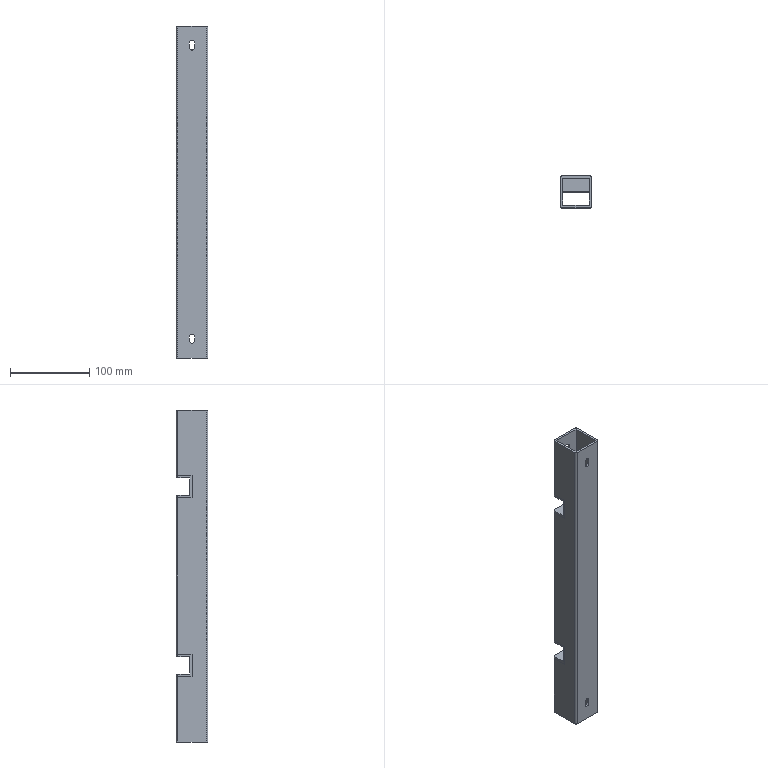Part | STEP file | X77-09106 | 3 solids | 78 faces | box 40 x 40 x 420 mm | volume 186089 mm3 | plane 50 | cylinder 28 | commonest cylinder face diameters 4 x16 6.5 x6 12 x6